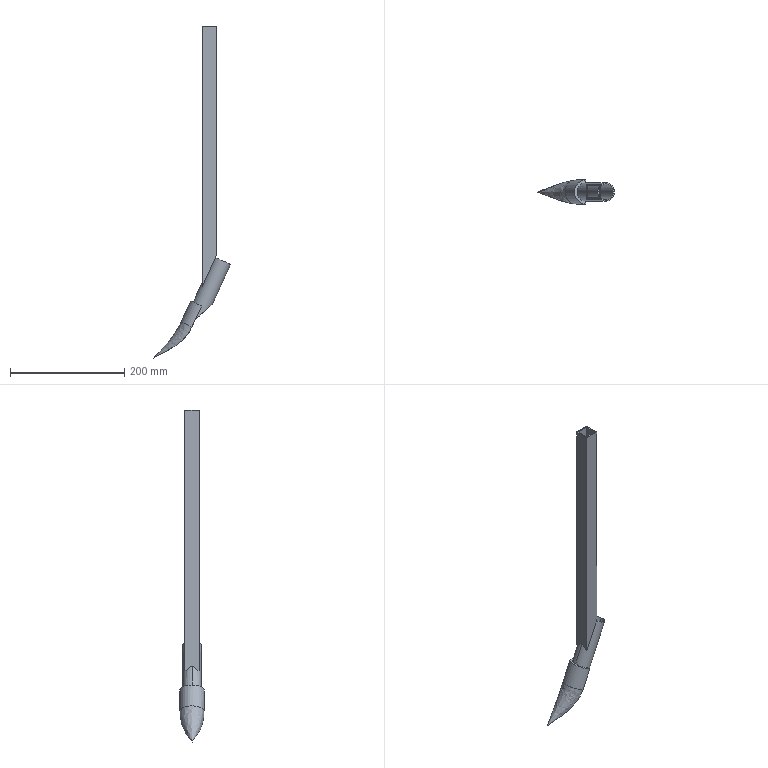Part | SolidWorks | features ICE 5, Blend 1, Extrusion 1 | 1 solid | 31 faces | box 134.332 x 42 x 580 mm | volume 122750 mm3 | plane 19 | cylinder 8 | spline 4 | commonest cylinder face diameters 32 x5 28 x2 42 x1
STEP:
#1=CARTESIAN_POINT('',(2.036,0.,-33.269));
#2=VERTEX_POINT('',#1);
#3=CARTESIAN_POINT('',(-50.61,0.,-81.426));
#4=VERTEX_POINT('',#3);
#5=CARTESIAN_POINT('',(2.036,0.,-33.269));
#6=CARTESIAN_POINT('',(2.036,-28.,-33.269));
#7=CARTESIAN_POINT('',(-50.61,-28.,-81.426));
#8=CARTESIAN_POINT('',(-50.61,0.,-81.426));
#9=(BOUNDED_CURVE()B_SPLINE_CURVE(3,(#5,#6,#7,#8),.UNSPECIFIED.,.F.,.F.)B_SPLINE_CURVE_WITH_KNOTS((4,4),(0.,3.142),.UNSPECIFIED.)CURVE()GEOMETRIC_REPRESENTATION_ITEM()RATIONAL_B_SPLINE_CURVE((1.,0.3333,0.3333,1.))REPRESENTATION_ITEM(''));
#10=EDGE_CURVE('',#2,#4,#9,.T.);
#11=ORIENTED_EDGE('',*,*,#10,.T.);
#12=CARTESIAN_POINT('',(-12.5,0.,2.417));
#13=VERTEX_POINT('',#12);
#14=CARTESIAN_POINT('',(-52.55,0.,-85.693));
#15=DIRECTION('',(0.4138,0.,0.9104));
#16=VECTOR('',#15,1000.);
#17=LINE('',#14,#16);
#18=EDGE_CURVE('',#4,#13,#17,.T.);
#19=ORIENTED_EDGE('',*,*,#18,.T.);
#20=CARTESIAN_POINT('',(-12.5,-3.14,1.555));
#21=VERTEX_POINT('',#20);
#22=CARTESIAN_POINT('',(-12.5,0.,2.417));
#23=CARTESIAN_POINT('',(-12.5,-1.058,2.417));
#24=CARTESIAN_POINT('',(-12.5,-2.109,2.128));
#25=CARTESIAN_POINT('',(-12.5,-3.14,1.555));
#26=(BOUNDED_CURVE()B_SPLINE_CURVE(3,(#22,#23,#24,#25),.UNSPECIFIED.,.F.,.T.)B_SPLINE_CURVE_WITH_KNOTS((4,4),(0.,0.2262),.UNSPECIFIED.)CURVE()GEOMETRIC_REPRESENTATION_ITEM()RATIONAL_B_SPLINE_CURVE((1.,0.9957,0.9957,1.))REPRESENTATION_ITEM(''));
#27=EDGE_CURVE('',#13,#21,#26,.T.);
#28=ORIENTED_EDGE('',*,*,#27,.T.);
#29=CARTESIAN_POINT('',(-11.914,-5.196,1.288));
#30=VERTEX_POINT('',#29);
#31=CARTESIAN_POINT('',(-0.07961,0.,-4.091));
#32=DIRECTION('',(-0.4138,0.,-0.9104));
#33=DIRECTION('',(-0.9104,0.,0.4138));
#34=AXIS2_PLACEMENT_3D('',#31,#32,#33);
#35=CIRCLE('',#34,14.);
#36=EDGE_CURVE('',#30,#21,#35,.T.);
#37=ORIENTED_EDGE('',*,*,#36,.F.);
#38=CARTESIAN_POINT('',(-10.5,-5.196,4.4));
#39=VERTEX_POINT('',#38);
#40=CARTESIAN_POINT('',(-51.639,-5.196,-86.107));
#41=DIRECTION('',(0.4138,0.,0.9104));
#42=VECTOR('',#41,1000.);
#43=LINE('',#40,#42);
#44=EDGE_CURVE('',#30,#39,#43,.T.);
#45=ORIENTED_EDGE('',*,*,#44,.T.);
#46=CARTESIAN_POINT('',(-10.5,0.,6.817));
#47=VERTEX_POINT('',#46);
#48=CARTESIAN_POINT('',(-10.5,0.,6.817));
#49=CARTESIAN_POINT('',(-10.5,-1.785,6.817));
#50=CARTESIAN_POINT('',(-10.5,-3.538,6.001));
#51=CARTESIAN_POINT('',(-10.5,-5.196,4.4));
#52=(BOUNDED_CURVE()B_SPLINE_CURVE(3,(#48,#49,#50,#51),.UNSPECIFIED.,.F.,.F.)B_SPLINE_CURVE_WITH_KNOTS((4,4),(0.,0.3803),.UNSPECIFIED.)CURVE()GEOMETRIC_REPRESENTATION_ITEM()RATIONAL_B_SPLINE_CURVE((1.,0.988,0.988,1.))REPRESENTATION_ITEM(''));
#53=EDGE_CURVE('',#47,#39,#52,.T.);
#54=ORIENTED_EDGE('',*,*,#53,.F.);
#55=CARTESIAN_POINT('',(9.521,0.,50.862));
#56=VERTEX_POINT('',#55);
#57=CARTESIAN_POINT('',(-52.55,0.,-85.693));
#58=DIRECTION('',(0.4138,0.,0.9104));
#59=VECTOR('',#58,1000.);
#60=LINE('',#57,#59);
#61=EDGE_CURVE('',#47,#56,#60,.T.);
#62=ORIENTED_EDGE('',*,*,#61,.T.);
#63=CARTESIAN_POINT('',(35.011,0.,39.275));
#64=VERTEX_POINT('',#63);
#65=CARTESIAN_POINT('',(22.266,0.,45.069));
#66=DIRECTION('',(0.4138,0.,0.9104));
#67=DIRECTION('',(0.9104,0.,-0.4138));
#68=AXIS2_PLACEMENT_3D('',#65,#66,#67);
#69=CIRCLE('',#68,14.);
#70=EDGE_CURVE('',#56,#64,#69,.T.);
#71=ORIENTED_EDGE('',*,*,#70,.T.);
#72=CARTESIAN_POINT('',(-27.06,0.,-97.279));
#73=DIRECTION('',(0.4138,0.,0.9104));
#74=VECTOR('',#73,1000.);
#75=LINE('',#72,#74);
#76=EDGE_CURVE('',#2,#64,#75,.T.);
#77=ORIENTED_EDGE('',*,*,#76,.F.);
#78=EDGE_LOOP('',(#11,#19,#28,#37,#45,#54,#62,#71,#77));
#79=FACE_OUTER_BOUND('',#78,.T.);
#80=CARTESIAN_POINT('',(-39.805,0.,-91.486));
#81=DIRECTION('',(0.4138,0.,0.9104));
#82=DIRECTION('',(0.9104,0.,-0.4138));
#83=AXIS2_PLACEMENT_3D('',#80,#81,#82);
#84=CYLINDRICAL_SURFACE('',#83,14.);
#85=ADVANCED_FACE('',(#79),#84,.F.);
#86=CARTESIAN_POINT('',(-28.301,0.,-27.512));
#87=VERTEX_POINT('',#86);
#88=CARTESIAN_POINT('',(-13.735,16.,-34.133));
#89=VERTEX_POINT('',#88);
#90=CARTESIAN_POINT('',(-13.735,0.,-34.133));
#91=DIRECTION('',(-0.4138,0.,-0.9104));
#92=DIRECTION('',(0.9104,0.,-0.4138));
#93=AXIS2_PLACEMENT_3D('',#90,#91,#92);
#94=CIRCLE('',#93,16.);
#95=EDGE_CURVE('',#87,#89,#94,.T.);
#96=ORIENTED_EDGE('',*,*,#95,.F.);
#97=CARTESIAN_POINT('',(-12.5,0.,7.25));
#98=VERTEX_POINT('',#97);
#99=CARTESIAN_POINT('',(-54.371,0.,-84.865));
#100=DIRECTION('',(0.4138,0.,0.9104));
#101=VECTOR('',#100,1000.);
#102=LINE('',#99,#101);
#103=EDGE_CURVE('',#87,#98,#102,.T.);
#104=ORIENTED_EDGE('',*,*,#103,.T.);
#105=CARTESIAN_POINT('',(-12.5,9.327,0.));
#106=VERTEX_POINT('',#105);
#107=CARTESIAN_POINT('',(-12.5,9.327,0.));
#108=CARTESIAN_POINT('',(-12.5,6.586,4.753));
#109=CARTESIAN_POINT('',(-12.5,3.374,7.25));
#110=CARTESIAN_POINT('',(-12.5,0.,7.25));
#111=(BOUNDED_CURVE()B_SPLINE_CURVE(3,(#107,#108,#109,#110),.UNSPECIFIED.,.F.,.F.)B_SPLINE_CURVE_WITH_KNOTS((4,4),(5.661,6.283),.UNSPECIFIED.)CURVE()GEOMETRIC_REPRESENTATION_ITEM()RATIONAL_B_SPLINE_CURVE((1.,0.968,0.968,1.))REPRESENTATION_ITEM(''));
#112=EDGE_CURVE('',#106,#98,#111,.T.);
#113=ORIENTED_EDGE('',*,*,#112,.F.);
#114=CARTESIAN_POINT('',(-10.5,9.327,4.4));
#115=VERTEX_POINT('',#114);
#116=CARTESIAN_POINT('',(-51.639,9.327,-86.107));
#117=DIRECTION('',(-0.4138,0.,-0.9104));
#118=VECTOR('',#117,1000.);
#119=LINE('',#116,#118);
#120=EDGE_CURVE('',#115,#106,#119,.T.);
#121=ORIENTED_EDGE('',*,*,#120,.F.);
#122=CARTESIAN_POINT('',(-10.5,0.,11.65));
#123=VERTEX_POINT('',#122);
#124=CARTESIAN_POINT('',(-10.5,9.327,4.4));
#125=CARTESIAN_POINT('',(-10.5,6.586,9.153));
#126=CARTESIAN_POINT('',(-10.5,3.374,11.65));
#127=CARTESIAN_POINT('',(-10.5,0.,11.65));
#128=(BOUNDED_CURVE()B_SPLINE_CURVE(3,(#124,#125,#126,#127),.UNSPECIFIED.,.F.,.F.)B_SPLINE_CURVE_WITH_KNOTS((4,4),(5.661,6.283),.UNSPECIFIED.)CURVE()GEOMETRIC_REPRESENTATION_ITEM()RATIONAL_B_SPLINE_CURVE((1.,0.968,0.968,1.))REPRESENTATION_ITEM(''));
#129=EDGE_CURVE('',#115,#123,#128,.T.);
#130=ORIENTED_EDGE('',*,*,#129,.T.);
#131=CARTESIAN_POINT('',(7.7,0.,51.69));
#132=VERTEX_POINT('',#131);
#133=CARTESIAN_POINT('',(-54.371,0.,-84.865));
#134=DIRECTION('',(0.4138,0.,0.9104));
#135=VECTOR('',#134,1000.);
#136=LINE('',#133,#135);
#137=EDGE_CURVE('',#123,#132,#136,.T.);
#138=ORIENTED_EDGE('',*,*,#137,.T.);
#139=CARTESIAN_POINT('',(36.832,0.,38.448));
#140=VERTEX_POINT('',#139);
#141=CARTESIAN_POINT('',(22.266,0.,45.069));
#142=DIRECTION('',(0.4138,0.,0.9104));
#143=DIRECTION('',(0.9104,0.,-0.4138));
#144=AXIS2_PLACEMENT_3D('',#141,#142,#143);
#145=CIRCLE('',#144,16.);
#146=EDGE_CURVE('',#140,#132,#145,.T.);
#147=ORIENTED_EDGE('',*,*,#146,.F.);
#148=CARTESIAN_POINT('',(5.796,0.,-29.83));
#149=VERTEX_POINT('',#148);
#150=CARTESIAN_POINT('',(-25.239,0.,-98.107));
#151=DIRECTION('',(0.4138,0.,0.9104));
#152=VECTOR('',#151,1000.);
#153=LINE('',#150,#152);
#154=EDGE_CURVE('',#149,#140,#153,.T.);
#155=ORIENTED_EDGE('',*,*,#154,.F.);
#156=CARTESIAN_POINT('',(-24.287,16.,-57.347));
#157=VERTEX_POINT('',#156);
#158=CARTESIAN_POINT('',(-24.287,16.,-57.347));
#159=CARTESIAN_POINT('',(-6.665,16.,-41.228));
#160=CARTESIAN_POINT('',(5.796,9.373,-29.83));
#161=CARTESIAN_POINT('',(5.796,0.,-29.83));
#162=(BOUNDED_CURVE()B_SPLINE_CURVE(3,(#158,#159,#160,#161),.UNSPECIFIED.,.F.,.F.)B_SPLINE_CURVE_WITH_KNOTS((4,4),(4.712,6.283),.UNSPECIFIED.)CURVE()GEOMETRIC_REPRESENTATION_ITEM()RATIONAL_B_SPLINE_CURVE((1.,0.8047,0.8047,1.))REPRESENTATION_ITEM(''));
#163=EDGE_CURVE('',#157,#149,#162,.T.);
#164=ORIENTED_EDGE('',*,*,#163,.F.);
#165=CARTESIAN_POINT('',(-30.287,16.,-70.548));
#166=DIRECTION('',(0.4138,0.,0.9104));
#167=VECTOR('',#166,1000.);
#168=LINE('',#165,#167);
#169=EDGE_CURVE('',#157,#89,#168,.T.);
#170=ORIENTED_EDGE('',*,*,#169,.T.);
#171=EDGE_LOOP('',(#96,#104,#113,#121,#130,#138,#147,#155,#164,#170));
#172=FACE_OUTER_BOUND('',#171,.T.);
#173=CARTESIAN_POINT('',(-39.805,0.,-91.486));
#174=DIRECTION('',(0.4138,0.,0.9104));
#175=DIRECTION('',(0.9104,0.,-0.4138));
#176=AXIS2_PLACEMENT_3D('',#173,#174,#175);
#177=CYLINDRICAL_SURFACE('',#176,16.);
#178=ADVANCED_FACE('',(#172),#177,.T.);
#179=CARTESIAN_POINT('',(-37.266,14.434,-69.22));
#180=VERTEX_POINT('',#179);
#181=CARTESIAN_POINT('',(-36.571,14.434,-67.691));
#182=VERTEX_POINT('',#181);
#183=CARTESIAN_POINT('',(-37.266,14.434,-69.22));
#184=CARTESIAN_POINT('',(-37.035,14.434,-68.711));
#185=CARTESIAN_POINT('',(-36.803,14.434,-68.202));
#186=CARTESIAN_POINT('',(-36.571,14.434,-67.691));
#187=B_SPLINE_CURVE_WITH_KNOTS('',3,(#183,#184,#185,#186),.UNSPECIFIED.,.F.,.F.,(4,4),(0.8196,1.),.UNSPECIFIED.);
#188=EDGE_CURVE('',#180,#182,#187,.T.);
#189=ORIENTED_EDGE('',*,*,#188,.F.);
#190=CARTESIAN_POINT('',(-37.266,-14.434,-69.22));
#191=VERTEX_POINT('',#190);
#192=CARTESIAN_POINT('',(-37.266,-14.434,-69.22));
#193=CARTESIAN_POINT('',(-63.552,-7.748,-93.264));
#194=CARTESIAN_POINT('',(-63.552,7.748,-93.264));
#195=CARTESIAN_POINT('',(-37.266,14.434,-69.22));
#196=(BOUNDED_CURVE()B_SPLINE_CURVE(3,(#192,#193,#194,#195),.UNSPECIFIED.,.F.,.T.)B_SPLINE_CURVE_WITH_KNOTS((4,4),(2.017,4.266),.UNSPECIFIED.)CURVE()GEOMETRIC_REPRESENTATION_ITEM()RATIONAL_B_SPLINE_CURVE((1.,0.621,0.621,1.))REPRESENTATION_ITEM(''));
#197=EDGE_CURVE('',#191,#180,#196,.T.);
#198=ORIENTED_EDGE('',*,*,#197,.F.);
#199=CARTESIAN_POINT('',(-36.571,-14.434,-67.691));
#200=VERTEX_POINT('',#199);
#201=CARTESIAN_POINT('',(-37.266,-14.434,-69.22));
#202=CARTESIAN_POINT('',(-37.034,-14.434,-68.71));
#203=CARTESIAN_POINT('',(-36.803,-14.434,-68.201));
#204=CARTESIAN_POINT('',(-36.571,-14.434,-67.691));
#205=B_SPLINE_CURVE_WITH_KNOTS('',3,(#201,#202,#203,#204),.UNSPECIFIED.,.F.,.F.,(4,4),(0.8182,1.),.UNSPECIFIED.);
#206=EDGE_CURVE('',#191,#200,#205,.T.);
#207=ORIENTED_EDGE('',*,*,#206,.T.);
#208=CARTESIAN_POINT('',(-30.287,0.,-70.548));
#209=DIRECTION('',(0.4138,0.,0.9104));
#210=DIRECTION('',(-0.9104,0.,0.4138));
#211=AXIS2_PLACEMENT_3D('',#208,#209,#210);
#212=CIRCLE('',#211,16.);
#213=EDGE_CURVE('',#182,#200,#212,.T.);
#214=ORIENTED_EDGE('',*,*,#213,.F.);
#215=EDGE_LOOP('',(#189,#198,#207,#214));
#216=FACE_OUTER_BOUND('',#215,.T.);
#217=CARTESIAN_POINT('',(-39.805,0.,-91.486));
#218=DIRECTION('',(0.4138,0.,0.9104));
#219=DIRECTION('',(0.9104,0.,-0.4138));
#220=AXIS2_PLACEMENT_3D('',#217,#218,#219);
#221=CYLINDRICAL_SURFACE('',#220,16.);
#222=ADVANCED_FACE('',(#216),#221,.T.);
#223=CARTESIAN_POINT('',(-11.914,5.196,1.288));
#224=VERTEX_POINT('',#223);
#225=CARTESIAN_POINT('',(-11.914,-202.5,1.288));
#226=DIRECTION('',(0.,-1.,0.));
#227=VECTOR('',#226,1000.);
#228=LINE('',#225,#227);
#229=EDGE_CURVE('',#224,#30,#228,.T.);
#230=ORIENTED_EDGE('',*,*,#229,.F.);
#231=CARTESIAN_POINT('',(-10.5,5.196,4.4));
#232=VERTEX_POINT('',#231);
#233=CARTESIAN_POINT('',(-51.639,5.196,-86.107));
#234=DIRECTION('',(-0.4138,0.,-0.9104));
#235=VECTOR('',#234,1000.);
#236=LINE('',#233,#235);
#237=EDGE_CURVE('',#232,#224,#236,.T.);
#238=ORIENTED_EDGE('',*,*,#237,.F.);
#239=CARTESIAN_POINT('',(-10.5,-10.5,4.4));
#240=DIRECTION('',(0.,-1.,0.));
#241=VECTOR('',#240,1000.);
#242=LINE('',#239,#241);
#243=EDGE_CURVE('',#232,#39,#242,.T.);
#244=ORIENTED_EDGE('',*,*,#243,.T.);
#245=ORIENTED_EDGE('',*,*,#44,.F.);
#246=EDGE_LOOP('',(#230,#238,#244,#245));
#247=FACE_OUTER_BOUND('',#246,.T.);
#248=CARTESIAN_POINT('',(-12.5,-202.5,0.));
#249=DIRECTION('',(-0.9104,0.,0.4138));
#250=DIRECTION('',(0.4138,0.,0.9104));
#251=AXIS2_PLACEMENT_3D('',#248,#249,#250);
#252=PLANE('',#251);
#253=ADVANCED_FACE('',(#247),#252,.F.);
#254=CARTESIAN_POINT('',(-12.5,3.14,1.555));
#255=VERTEX_POINT('',#254);
#256=CARTESIAN_POINT('',(-12.5,-12.5,1.555));
#257=DIRECTION('',(0.,1.,0.));
#258=VECTOR('',#257,1000.);
#259=LINE('',#256,#258);
#260=EDGE_CURVE('',#21,#255,#259,.T.);
#261=ORIENTED_EDGE('',*,*,#260,.F.);
#262=ORIENTED_EDGE('',*,*,#27,.F.);
#263=CARTESIAN_POINT('',(-12.5,3.14,1.555));
#264=CARTESIAN_POINT('',(-12.5,2.109,2.128));
#265=CARTESIAN_POINT('',(-12.5,1.058,2.417));
#266=CARTESIAN_POINT('',(-12.5,0.,2.417));
#267=(BOUNDED_CURVE()B_SPLINE_CURVE(3,(#263,#264,#265,#266),.UNSPECIFIED.,.F.,.F.)B_SPLINE_CURVE_WITH_KNOTS((4,4),(6.057,6.283),.UNSPECIFIED.)CURVE()GEOMETRIC_REPRESENTATION_ITEM()RATIONAL_B_SPLINE_CURVE((1.,0.9957,0.9957,1.))REPRESENTATION_ITEM(''));
#268=EDGE_CURVE('',#255,#13,#267,.T.);
#269=ORIENTED_EDGE('',*,*,#268,.F.);
#270=EDGE_LOOP('',(#261,#262,#269));
#271=FACE_OUTER_BOUND('',#270,.T.);
#272=CARTESIAN_POINT('',(-12.5,-12.5,455.));
#273=DIRECTION('',(1.,0.,0.));
#274=DIRECTION('',(0.,0.,-1.));
#275=AXIS2_PLACEMENT_3D('',#272,#273,#274);
#276=PLANE('',#275);
#277=ADVANCED_FACE('',(#271),#276,.F.);
#278=CARTESIAN_POINT('',(-12.5,12.5,455.));
#279=VERTEX_POINT('',#278);
#280=CARTESIAN_POINT('',(-12.5,-12.5,455.));
#281=VERTEX_POINT('',#280);
#282=CARTESIAN_POINT('',(-12.5,-12.5,455.));
#283=DIRECTION('',(0.,-1.,0.));
#284=VECTOR('',#283,1000.);
#285=LINE('',#282,#284);
#286=EDGE_CURVE('',#279,#281,#285,.T.);
#287=ORIENTED_EDGE('',*,*,#286,.T.);
#288=CARTESIAN_POINT('',(12.5,-12.5,455.));
#289=VERTEX_POINT('',#288);
#290=CARTESIAN_POINT('',(12.5,-12.5,455.));
#291=DIRECTION('',(1.,0.,0.));
#292=VECTOR('',#291,1000.);
#293=LINE('',#290,#292);
#294=EDGE_CURVE('',#281,#289,#293,.T.);
#295=ORIENTED_EDGE('',*,*,#294,.T.);
#296=CARTESIAN_POINT('',(12.5,12.5,455.));
#297=VERTEX_POINT('',#296);
#298=CARTESIAN_POINT('',(12.5,-12.5,455.));
#299=DIRECTION('',(0.,1.,0.));
#300=VECTOR('',#299,1000.);
#301=LINE('',#298,#300);
#302=EDGE_CURVE('',#289,#297,#301,.T.);
#303=ORIENTED_EDGE('',*,*,#302,.T.);
#304=CARTESIAN_POINT('',(12.5,12.5,455.));
#305=DIRECTION('',(-1.,0.,0.));
#306=VECTOR('',#305,1000.);
#307=LINE('',#304,#306);
#308=EDGE_CURVE('',#297,#279,#307,.T.);
#309=ORIENTED_EDGE('',*,*,#308,.T.);
#310=EDGE_LOOP('',(#287,#295,#303,#309));
#311=FACE_OUTER_BOUND('',#310,.T.);
#312=CARTESIAN_POINT('',(-10.5,-10.5,455.));
#313=VERTEX_POINT('',#312);
#314=CARTESIAN_POINT('',(10.5,-10.5,455.));
#315=VERTEX_POINT('',#314);
#316=CARTESIAN_POINT('',(10.5,-10.5,455.));
#317=DIRECTION('',(1.,0.,0.));
#318=VECTOR('',#317,1000.);
#319=LINE('',#316,#318);
#320=EDGE_CURVE('',#313,#315,#319,.T.);
#321=ORIENTED_EDGE('',*,*,#320,.F.);
#322=CARTESIAN_POINT('',(-10.5,10.5,455.));
#323=VERTEX_POINT('',#322);
#324=CARTESIAN_POINT('',(-10.5,-10.5,455.));
#325=DIRECTION('',(0.,-1.,0.));
#326=VECTOR('',#325,1000.);
#327=LINE('',#324,#326);
#328=EDGE_CURVE('',#323,#313,#327,.T.);
#329=ORIENTED_EDGE('',*,*,#328,.F.);
#330=CARTESIAN_POINT('',(10.5,10.5,455.));
#331=VERTEX_POINT('',#330);
#332=CARTESIAN_POINT('',(10.5,10.5,455.));
#333=DIRECTION('',(-1.,0.,0.));
#334=VECTOR('',#333,1000.);
#335=LINE('',#332,#334);
#336=EDGE_CURVE('',#331,#323,#335,.T.);
#337=ORIENTED_EDGE('',*,*,#336,.F.);
#338=CARTESIAN_POINT('',(10.5,-10.5,455.));
#339=DIRECTION('',(0.,1.,0.));
#340=VECTOR('',#339,1000.);
#341=LINE('',#338,#340);
#342=EDGE_CURVE('',#315,#331,#341,.T.);
#343=ORIENTED_EDGE('',*,*,#342,.F.);
#344=EDGE_LOOP('',(#321,#329,#337,#343));
#345=FACE_BOUND('',#344,.T.);
#346=CARTESIAN_POINT('',(0.,0.,455.));
#347=DIRECTION('',(0.,0.,1.));
#348=DIRECTION('',(1.,0.,0.));
#349=AXIS2_PLACEMENT_3D('',#346,#347,#348);
#350=PLANE('',#349);
#351=ADVANCED_FACE('',(#311,#345),#350,.T.);
#352=CARTESIAN_POINT('',(-12.5,12.5,0.));
#353=VERTEX_POINT('',#352);
#354=CARTESIAN_POINT('',(-12.5,-12.5,0.));
#355=DIRECTION('',(0.,-1.,0.));
#356=VECTOR('',#355,1000.);
#357=LINE('',#354,#356);
#358=EDGE_CURVE('',#353,#106,#357,.T.);
#359=ORIENTED_EDGE('',*,*,#358,.T.);
#360=ORIENTED_EDGE('',*,*,#112,.T.);
#361=CARTESIAN_POINT('',(-12.5,-9.327,0.));
#362=VERTEX_POINT('',#361);
#363=CARTESIAN_POINT('',(-12.5,0.,7.25));
#364=CARTESIAN_POINT('',(-12.5,-3.374,7.25));
#365=CARTESIAN_POINT('',(-12.5,-6.586,4.753));
#366=CARTESIAN_POINT('',(-12.5,-9.327,0.));
#367=(BOUNDED_CURVE()B_SPLINE_CURVE(3,(#363,#364,#365,#366),.UNSPECIFIED.,.F.,.T.)B_SPLINE_CURVE_WITH_KNOTS((4,4),(0.,0.6224),.UNSPECIFIED.)CURVE()GEOMETRIC_REPRESENTATION_ITEM()RATIONAL_B_SPLINE_CURVE((1.,0.968,0.968,1.))REPRESENTATION_ITEM(''));
#368=EDGE_CURVE('',#98,#362,#367,.T.);
#369=ORIENTED_EDGE('',*,*,#368,.T.);
#370=CARTESIAN_POINT('',(-12.5,-12.5,0.));
#371=VERTEX_POINT('',#370);
#372=CARTESIAN_POINT('',(-12.5,-12.5,0.));
#373=DIRECTION('',(0.,-1.,0.));
#374=VECTOR('',#373,1000.);
#375=LINE('',#372,#374);
#376=EDGE_CURVE('',#362,#371,#375,.T.);
#377=ORIENTED_EDGE('',*,*,#376,.T.);
#378=CARTESIAN_POINT('',(-12.5,-12.5,455.));
#379=DIRECTION('',(0.,0.,-1.));
#380=VECTOR('',#379,1000.);
#381=LINE('',#378,#380);
#382=EDGE_CURVE('',#281,#371,#381,.T.);
#383=ORIENTED_EDGE('',*,*,#382,.F.);
#384=ORIENTED_EDGE('',*,*,#286,.F.);
#385=CARTESIAN_POINT('',(-12.5,12.5,455.));
#386=DIRECTION('',(0.,0.,-1.));
#387=VECTOR('',#386,1000.);
#388=LINE('',#385,#387);
#389=EDGE_CURVE('',#279,#353,#388,.T.);
#390=ORIENTED_EDGE('',*,*,#389,.T.);
#391=EDGE_LOOP('',(#359,#360,#369,#377,#383,#384,#390));
#392=FACE_OUTER_BOUND('',#391,.T.);
#393=CARTESIAN_POINT('',(-12.5,-12.5,455.));
#394=DIRECTION('',(1.,0.,0.));
#395=DIRECTION('',(0.,0.,-1.));
#396=AXIS2_PLACEMENT_3D('',#393,#394,#395);
#397=PLANE('',#396);
#398=ADVANCED_FACE('',(#392),#397,.F.);
#399=ORIENTED_EDGE('',*,*,#382,.T.);
#400=CARTESIAN_POINT('',(12.5,-12.5,55.));
#401=VERTEX_POINT('',#400);
#402=CARTESIAN_POINT('',(163.185,-12.5,386.507));
#403=DIRECTION('',(0.4138,0.,0.9104));
#404=VECTOR('',#403,1000.);
#405=LINE('',#402,#404);
#406=EDGE_CURVE('',#371,#401,#405,.T.);
#407=ORIENTED_EDGE('',*,*,#406,.T.);
#408=CARTESIAN_POINT('',(12.5,-12.5,455.));
#409=DIRECTION('',(0.,0.,-1.));
#410=VECTOR('',#409,1000.);
#411=LINE('',#408,#410);
#412=EDGE_CURVE('',#289,#401,#411,.T.);
#413=ORIENTED_EDGE('',*,*,#412,.F.);
#414=ORIENTED_EDGE('',*,*,#294,.F.);
#415=EDGE_LOOP('',(#399,#407,#413,#414));
#416=FACE_OUTER_BOUND('',#415,.T.);
#417=CARTESIAN_POINT('',(12.5,-12.5,455.));
#418=DIRECTION('',(0.,1.,0.));
#419=DIRECTION('',(-1.,0.,0.));
#420=AXIS2_PLACEMENT_3D('',#417,#418,#419);
#421=PLANE('',#420);
#422=ADVANCED_FACE('',(#416),#421,.F.);
#423=ORIENTED_EDGE('',*,*,#412,.T.);
#424=CARTESIAN_POINT('',(12.5,12.5,55.));
#425=VERTEX_POINT('',#424);
#426=CARTESIAN_POINT('',(12.5,-202.5,55.));
#427=DIRECTION('',(0.,1.,0.));
#428=VECTOR('',#427,1000.);
#429=LINE('',#426,#428);
#430=EDGE_CURVE('',#401,#425,#429,.T.);
#431=ORIENTED_EDGE('',*,*,#430,.T.);
#432=CARTESIAN_POINT('',(12.5,12.5,455.));
#433=DIRECTION('',(0.,0.,-1.));
#434=VECTOR('',#433,1000.);
#435=LINE('',#432,#434);
#436=EDGE_CURVE('',#297,#425,#435,.T.);
#437=ORIENTED_EDGE('',*,*,#436,.F.);
#438=ORIENTED_EDGE('',*,*,#302,.F.);
#439=EDGE_LOOP('',(#423,#431,#437,#438));
#440=FACE_OUTER_BOUND('',#439,.T.);
#441=CARTESIAN_POINT('',(12.5,-12.5,455.));
#442=DIRECTION('',(-1.,0.,0.));
#443=DIRECTION('',(0.,0.,1.));
#444=AXIS2_PLACEMENT_3D('',#441,#442,#443);
#445=PLANE('',#444);
#446=ADVANCED_FACE('',(#440),#445,.F.);
#447=ORIENTED_EDGE('',*,*,#436,.T.);
#448=CARTESIAN_POINT('',(-12.5,12.5,0.));
#449=DIRECTION('',(0.4138,0.,0.9104));
#450=VECTOR('',#449,1000.);
#451=LINE('',#448,#450);
#452=EDGE_CURVE('',#353,#425,#451,.T.);
#453=ORIENTED_EDGE('',*,*,#452,.F.);
#454=ORIENTED_EDGE('',*,*,#389,.F.);
#455=ORIENTED_EDGE('',*,*,#308,.F.);
#456=EDGE_LOOP('',(#447,#453,#454,#455));
#457=FACE_OUTER_BOUND('',#456,.T.);
#458=CARTESIAN_POINT('',(12.5,12.5,455.));
#459=DIRECTION('',(0.,-1.,0.));
#460=DIRECTION('',(1.,0.,0.));
#461=AXIS2_PLACEMENT_3D('',#458,#459,#460);
#462=PLANE('',#461);
#463=ADVANCED_FACE('',(#457),#462,.F.);
#464=ORIENTED_EDGE('',*,*,#129,.F.);
#465=CARTESIAN_POINT('',(-10.5,10.5,4.4));
#466=VERTEX_POINT('',#465);
#467=CARTESIAN_POINT('',(-10.5,-10.5,4.4));
#468=DIRECTION('',(0.,-1.,0.));
#469=VECTOR('',#468,1000.);
#470=LINE('',#467,#469);
#471=EDGE_CURVE('',#466,#115,#470,.T.);
#472=ORIENTED_EDGE('',*,*,#471,.F.);
#473=CARTESIAN_POINT('',(-10.5,10.5,455.));
#474=DIRECTION('',(0.,0.,-1.));
#475=VECTOR('',#474,1000.);
#476=LINE('',#473,#475);
#477=EDGE_CURVE('',#323,#466,#476,.T.);
#478=ORIENTED_EDGE('',*,*,#477,.F.);
#479=ORIENTED_EDGE('',*,*,#328,.T.);
#480=CARTESIAN_POINT('',(-10.5,-10.5,4.4));
#481=VERTEX_POINT('',#480);
#482=CARTESIAN_POINT('',(-10.5,-10.5,455.));
#483=DIRECTION('',(0.,0.,-1.));
#484=VECTOR('',#483,1000.);
#485=LINE('',#482,#484);
#486=EDGE_CURVE('',#313,#481,#485,.T.);
#487=ORIENTED_EDGE('',*,*,#486,.T.);
#488=CARTESIAN_POINT('',(-10.5,-9.327,4.4));
#489=VERTEX_POINT('',#488);
#490=CARTESIAN_POINT('',(-10.5,-10.5,4.4));
#491=DIRECTION('',(0.,-1.,0.));
#492=VECTOR('',#491,1000.);
#493=LINE('',#490,#492);
#494=EDGE_CURVE('',#489,#481,#493,.T.);
#495=ORIENTED_EDGE('',*,*,#494,.F.);
#496=CARTESIAN_POINT('',(-10.5,0.,11.65));
#497=CARTESIAN_POINT('',(-10.5,-3.374,11.65));
#498=CARTESIAN_POINT('',(-10.5,-6.586,9.153));
#499=CARTESIAN_POINT('',(-10.5,-9.327,4.4));
#500=(BOUNDED_CURVE()B_SPLINE_CURVE(3,(#496,#497,#498,#499),.UNSPECIFIED.,.F.,.F.)B_SPLINE_CURVE_WITH_KNOTS((4,4),(0.,0.6224),.UNSPECIFIED.)CURVE()GEOMETRIC_REPRESENTATION_ITEM()RATIONAL_B_SPLINE_CURVE((1.,0.968,0.968,1.))REPRESENTATION_ITEM(''));
#501=EDGE_CURVE('',#123,#489,#500,.T.);
#502=ORIENTED_EDGE('',*,*,#501,.F.);
#503=EDGE_LOOP('',(#464,#472,#478,#479,#487,#495,#502));
#504=FACE_OUTER_BOUND('',#503,.T.);
#505=CARTESIAN_POINT('',(-10.5,-10.5,455.));
#506=DIRECTION('',(1.,0.,0.));
#507=DIRECTION('',(0.,1.,0.));
#508=AXIS2_PLACEMENT_3D('',#505,#506,#507);
#509=PLANE('',#508);
#510=ADVANCED_FACE('',(#504),#509,.T.);
#511=CARTESIAN_POINT('',(10.5,-10.5,50.6));
#512=VERTEX_POINT('',#511);
#513=CARTESIAN_POINT('',(162.842,-10.5,385.753));
#514=DIRECTION('',(0.4138,0.,0.9104));
#515=VECTOR('',#514,1000.);
#516=LINE('',#513,#515);
#517=EDGE_CURVE('',#481,#512,#516,.T.);
#518=ORIENTED_EDGE('',*,*,#517,.F.);
#519=ORIENTED_EDGE('',*,*,#486,.F.);
#520=ORIENTED_EDGE('',*,*,#320,.T.);
#521=CARTESIAN_POINT('',(10.5,-10.5,455.));
#522=DIRECTION('',(0.,0.,-1.));
#523=VECTOR('',#522,1000.);
#524=LINE('',#521,#523);
#525=EDGE_CURVE('',#315,#512,#524,.T.);
#526=ORIENTED_EDGE('',*,*,#525,.T.);
#527=EDGE_LOOP('',(#518,#519,#520,#526));
#528=FACE_OUTER_BOUND('',#527,.T.);
#529=CARTESIAN_POINT('',(10.5,-10.5,455.));
#530=DIRECTION('',(0.,1.,0.));
#531=DIRECTION('',(0.,0.,1.));
#532=AXIS2_PLACEMENT_3D('',#529,#530,#531);
#533=PLANE('',#532);
#534=ADVANCED_FACE('',(#528),#533,.T.);
#535=CARTESIAN_POINT('',(10.5,10.5,50.6));
#536=VERTEX_POINT('',#535);
#537=CARTESIAN_POINT('',(10.5,-10.5,50.6));
#538=DIRECTION('',(0.,1.,0.));
#539=VECTOR('',#538,1000.);
#540=LINE('',#537,#539);
#541=EDGE_CURVE('',#512,#536,#540,.T.);
#542=ORIENTED_EDGE('',*,*,#541,.F.);
#543=ORIENTED_EDGE('',*,*,#525,.F.);
#544=ORIENTED_EDGE('',*,*,#342,.T.);
#545=CARTESIAN_POINT('',(10.5,10.5,455.));
#546=DIRECTION('',(0.,0.,-1.));
#547=VECTOR('',#546,1000.);
#548=LINE('',#545,#547);
#549=EDGE_CURVE('',#331,#536,#548,.T.);
#550=ORIENTED_EDGE('',*,*,#549,.T.);
#551=EDGE_LOOP('',(#542,#543,#544,#550));
#552=FACE_OUTER_BOUND('',#551,.T.);
#553=CARTESIAN_POINT('',(10.5,-10.5,455.));
#554=DIRECTION('',(-1.,0.,0.));
#555=DIRECTION('',(0.,0.,1.));
#556=AXIS2_PLACEMENT_3D('',#553,#554,#555);
#557=PLANE('',#556);
#558=ADVANCED_FACE('',(#552),#557,.T.);
#559=CARTESIAN_POINT('',(162.842,10.5,385.753));
#560=DIRECTION('',(-0.4138,0.,-0.9104));
#561=VECTOR('',#560,1000.);
#562=LINE('',#559,#561);
#563=EDGE_CURVE('',#536,#466,#562,.T.);
#564=ORIENTED_EDGE('',*,*,#563,.F.);
#565=ORIENTED_EDGE('',*,*,#549,.F.);
#566=ORIENTED_EDGE('',*,*,#336,.T.);
#567=ORIENTED_EDGE('',*,*,#477,.T.);
#568=EDGE_LOOP('',(#564,#565,#566,#567));
#569=FACE_OUTER_BOUND('',#568,.T.);
#570=CARTESIAN_POINT('',(10.5,10.5,455.));
#571=DIRECTION('',(0.,-1.,0.));
#572=DIRECTION('',(1.,0.,0.));
#573=AXIS2_PLACEMENT_3D('',#570,#571,#572);
#574=PLANE('',#573);
#575=ADVANCED_FACE('',(#569),#574,.T.);
#576=ORIENTED_EDGE('',*,*,#376,.F.);
#577=CARTESIAN_POINT('',(-51.639,-9.327,-86.107));
#578=DIRECTION('',(0.4138,0.,0.9104));
#579=VECTOR('',#578,1000.);
#580=LINE('',#577,#579);
#581=EDGE_CURVE('',#362,#489,#580,.T.);
#582=ORIENTED_EDGE('',*,*,#581,.T.);
#583=ORIENTED_EDGE('',*,*,#494,.T.);
#584=ORIENTED_EDGE('',*,*,#517,.T.);
#585=ORIENTED_EDGE('',*,*,#541,.T.);
#586=ORIENTED_EDGE('',*,*,#563,.T.);
#587=ORIENTED_EDGE('',*,*,#471,.T.);
#588=ORIENTED_EDGE('',*,*,#120,.T.);
#589=ORIENTED_EDGE('',*,*,#358,.F.);
#590=ORIENTED_EDGE('',*,*,#452,.T.);
#591=ORIENTED_EDGE('',*,*,#430,.F.);
#592=ORIENTED_EDGE('',*,*,#406,.F.);
#593=EDGE_LOOP('',(#576,#582,#583,#584,#585,#586,#587,#588,#589,#590,#591,#592));
#594=FACE_OUTER_BOUND('',#593,.T.);
#595=CARTESIAN_POINT('',(-12.5,-202.5,0.));
#596=DIRECTION('',(-0.9104,0.,0.4138));
#597=DIRECTION('',(0.4138,0.,0.9104));
#598=AXIS2_PLACEMENT_3D('',#595,#596,#597);
#599=PLANE('',#598);
#600=ADVANCED_FACE('',(#594),#599,.F.);
#601=ORIENTED_EDGE('',*,*,#103,.F.);
#602=CARTESIAN_POINT('',(-13.735,-16.,-34.133));
#603=VERTEX_POINT('',#602);
#604=CARTESIAN_POINT('',(-13.735,0.,-34.133));
#605=DIRECTION('',(-0.4138,0.,-0.9104));
#606=DIRECTION('',(0.9104,0.,-0.4138));
#607=AXIS2_PLACEMENT_3D('',#604,#605,#606);
#608=CIRCLE('',#607,16.);
#609=EDGE_CURVE('',#603,#87,#608,.T.);
#610=ORIENTED_EDGE('',*,*,#609,.F.);
#611=CARTESIAN_POINT('',(-24.287,-16.,-57.347));
#612=VERTEX_POINT('',#611);
#613=CARTESIAN_POINT('',(-30.287,-16.,-70.548));
#614=DIRECTION('',(0.4138,0.,0.9104));
#615=VECTOR('',#614,1000.);
#616=LINE('',#613,#615);
#617=EDGE_CURVE('',#612,#603,#616,.T.);
#618=ORIENTED_EDGE('',*,*,#617,.F.);
#619=CARTESIAN_POINT('',(5.796,0.,-29.83));
#620=CARTESIAN_POINT('',(5.796,-9.373,-29.83));
#621=CARTESIAN_POINT('',(-6.665,-16.,-41.228));
#622=CARTESIAN_POINT('',(-24.287,-16.,-57.347));
#623=(BOUNDED_CURVE()B_SPLINE_CURVE(3,(#619,#620,#621,#622),.UNSPECIFIED.,.F.,.T.)B_SPLINE_CURVE_WITH_KNOTS((4,4),(0.,1.571),.UNSPECIFIED.)CURVE()GEOMETRIC_REPRESENTATION_ITEM()RATIONAL_B_SPLINE_CURVE((1.,0.8047,0.8047,1.))REPRESENTATION_ITEM(''));
#624=EDGE_CURVE('',#149,#612,#623,.T.);
#625=ORIENTED_EDGE('',*,*,#624,.F.);
#626=ORIENTED_EDGE('',*,*,#154,.T.);
#627=CARTESIAN_POINT('',(22.266,0.,45.069));
#628=DIRECTION('',(0.4138,0.,0.9104));
#629=DIRECTION('',(0.9104,0.,-0.4138));
#630=AXIS2_PLACEMENT_3D('',#627,#628,#629);
#631=CIRCLE('',#630,16.);
#632=EDGE_CURVE('',#132,#140,#631,.T.);
#633=ORIENTED_EDGE('',*,*,#632,.F.);
#634=ORIENTED_EDGE('',*,*,#137,.F.);
#635=ORIENTED_EDGE('',*,*,#501,.T.);
#636=ORIENTED_EDGE('',*,*,#581,.F.);
#637=ORIENTED_EDGE('',*,*,#368,.F.);
#638=EDGE_LOOP('',(#601,#610,#618,#625,#626,#633,#634,#635,#636,#637));
#639=FACE_OUTER_BOUND('',#638,.T.);
#640=CARTESIAN_POINT('',(-39.805,0.,-91.486));
#641=DIRECTION('',(0.4138,0.,0.9104));
#642=DIRECTION('',(0.9104,0.,-0.4138));
#643=AXIS2_PLACEMENT_3D('',#640,#641,#642);
#644=CYLINDRICAL_SURFACE('',#643,16.);
#645=ADVANCED_FACE('',(#639),#644,.T.);
#646=ORIENTED_EDGE('',*,*,#18,.F.);
#647=CARTESIAN_POINT('',(-50.61,0.,-81.426));
#648=CARTESIAN_POINT('',(-50.61,28.,-81.426));
#649=CARTESIAN_POINT('',(2.036,28.,-33.269));
#650=CARTESIAN_POINT('',(2.036,0.,-33.269));
#651=(BOUNDED_CURVE()B_SPLINE_CURVE(3,(#647,#648,#649,#650),.UNSPECIFIED.,.F.,.F.)B_SPLINE_CURVE_WITH_KNOTS((4,4),(3.142,6.283),.UNSPECIFIED.)CURVE()GEOMETRIC_REPRESENTATION_ITEM()RATIONAL_B_SPLINE_CURVE((1.,0.3333,0.3333,1.))REPRESENTATION_ITEM(''));
#652=EDGE_CURVE('',#4,#2,#651,.T.);
#653=ORIENTED_EDGE('',*,*,#652,.T.);
#654=ORIENTED_EDGE('',*,*,#76,.T.);
#655=CARTESIAN_POINT('',(22.266,0.,45.069));
#656=DIRECTION('',(0.4138,0.,0.9104));
#657=DIRECTION('',(0.9104,0.,-0.4138));
#658=AXIS2_PLACEMENT_3D('',#655,#656,#657);
#659=CIRCLE('',#658,14.);
#660=EDGE_CURVE('',#64,#56,#659,.T.);
#661=ORIENTED_EDGE('',*,*,#660,.T.);
#662=ORIENTED_EDGE('',*,*,#61,.F.);
#663=CARTESIAN_POINT('',(-10.5,5.196,4.4));
#664=CARTESIAN_POINT('',(-10.5,3.538,6.001));
#665=CARTESIAN_POINT('',(-10.5,1.785,6.817));
#666=CARTESIAN_POINT('',(-10.5,0.,6.817));
#667=(BOUNDED_CURVE()B_SPLINE_CURVE(3,(#663,#664,#665,#666),.UNSPECIFIED.,.F.,.F.)B_SPLINE_CURVE_WITH_KNOTS((4,4),(5.903,6.283),.UNSPECIFIED.)CURVE()GEOMETRIC_REPRESENTATION_ITEM()RATIONAL_B_SPLINE_CURVE((1.,0.988,0.988,1.))REPRESENTATION_ITEM(''));
#668=EDGE_CURVE('',#232,#47,#667,.T.);
#669=ORIENTED_EDGE('',*,*,#668,.F.);
#670=ORIENTED_EDGE('',*,*,#237,.T.);
#671=CARTESIAN_POINT('',(-0.07961,0.,-4.091));
#672=DIRECTION('',(-0.4138,0.,-0.9104));
#673=DIRECTION('',(-0.9104,0.,0.4138));
#674=AXIS2_PLACEMENT_3D('',#671,#672,#673);
#675=CIRCLE('',#674,14.);
#676=EDGE_CURVE('',#255,#224,#675,.T.);
#677=ORIENTED_EDGE('',*,*,#676,.F.);
#678=ORIENTED_EDGE('',*,*,#268,.T.);
#679=EDGE_LOOP('',(#646,#653,#654,#661,#662,#669,#670,#677,#678));
#680=FACE_OUTER_BOUND('',#679,.T.);
#681=CARTESIAN_POINT('',(-39.805,0.,-91.486));
#682=DIRECTION('',(0.4138,0.,0.9104));
#683=DIRECTION('',(0.9104,0.,-0.4138));
#684=AXIS2_PLACEMENT_3D('',#681,#682,#683);
#685=CYLINDRICAL_SURFACE('',#684,14.);
#686=ADVANCED_FACE('',(#680),#685,.F.);
#687=ORIENTED_EDGE('',*,*,#660,.F.);
#688=ORIENTED_EDGE('',*,*,#70,.F.);
#689=EDGE_LOOP('',(#687,#688));
#690=FACE_BOUND('',#689,.T.);
#691=ORIENTED_EDGE('',*,*,#146,.T.);
#692=ORIENTED_EDGE('',*,*,#632,.T.);
#693=EDGE_LOOP('',(#691,#692));
#694=FACE_OUTER_BOUND('',#693,.T.);
#695=CARTESIAN_POINT('',(22.266,0.,45.069));
#696=DIRECTION('',(0.4138,0.,0.9104));
#697=DIRECTION('',(0.9104,0.,-0.4138));
#698=AXIS2_PLACEMENT_3D('',#695,#696,#697);
#699=PLANE('',#698);
#700=ADVANCED_FACE('',(#690,#694),#699,.T.);
#701=ORIENTED_EDGE('',*,*,#243,.F.);
#702=ORIENTED_EDGE('',*,*,#668,.T.);
#703=ORIENTED_EDGE('',*,*,#53,.T.);
#704=EDGE_LOOP('',(#701,#702,#703));
#705=FACE_OUTER_BOUND('',#704,.T.);
#706=CARTESIAN_POINT('',(-10.5,-10.5,455.));
#707=DIRECTION('',(1.,0.,0.));
#708=DIRECTION('',(0.,1.,0.));
#709=AXIS2_PLACEMENT_3D('',#706,#707,#708);
#710=PLANE('',#709);
#711=ADVANCED_FACE('',(#705),#710,.T.);
#712=ORIENTED_EDGE('',*,*,#229,.T.);
#713=ORIENTED_EDGE('',*,*,#36,.T.);
#714=ORIENTED_EDGE('',*,*,#260,.T.);
#715=ORIENTED_EDGE('',*,*,#676,.T.);
#716=EDGE_LOOP('',(#712,#713,#714,#715));
#717=FACE_OUTER_BOUND('',#716,.T.);
#718=CARTESIAN_POINT('',(-0.07961,0.,-4.091));
#719=DIRECTION('',(-0.4138,0.,-0.9104));
#720=DIRECTION('',(-0.9104,0.,0.4138));
#721=AXIS2_PLACEMENT_3D('',#718,#719,#720);
#722=PLANE('',#721);
#723=ADVANCED_FACE('',(#717),#722,.T.);
#724=CARTESIAN_POINT('',(-36.872,14.533,-68.859));
#725=VERTEX_POINT('',#724);
#726=CARTESIAN_POINT('',(-37.266,14.434,-69.22));
#727=CARTESIAN_POINT('',(-37.135,14.468,-69.1));
#728=CARTESIAN_POINT('',(-37.004,14.5,-68.98));
#729=CARTESIAN_POINT('',(-36.872,14.533,-68.859));
#730=B_SPLINE_CURVE_WITH_KNOTS('',3,(#726,#727,#728,#729),.UNSPECIFIED.,.F.,.F.,(4,4),(0.,1.),.UNSPECIFIED.);
#731=EDGE_CURVE('',#180,#725,#730,.T.);
#732=ORIENTED_EDGE('',*,*,#731,.T.);
#733=CARTESIAN_POINT('',(-35.919,14.756,-67.988));
#734=VERTEX_POINT('',#733);
#735=CARTESIAN_POINT('',(-36.872,14.533,-68.859));
#736=CARTESIAN_POINT('',(-36.555,14.61,-68.569));
#737=CARTESIAN_POINT('',(-36.238,14.685,-68.279));
#738=CARTESIAN_POINT('',(-35.919,14.756,-67.988));
#739=B_SPLINE_CURVE_WITH_KNOTS('',3,(#735,#736,#737,#738),.UNSPECIFIED.,.F.,.F.,(4,4),(0.02512,0.02643),.UNSPECIFIED.);
#740=EDGE_CURVE('',#725,#734,#739,.T.);
#741=ORIENTED_EDGE('',*,*,#740,.T.);
#742=CARTESIAN_POINT('',(-35.919,14.756,-67.988));
#743=CARTESIAN_POINT('',(-32.224,15.58,-64.607));
#744=CARTESIAN_POINT('',(-28.295,16.,-61.013));
#745=CARTESIAN_POINT('',(-24.287,16.,-57.347));
#746=(BOUNDED_CURVE()B_SPLINE_CURVE(3,(#742,#743,#744,#745),.UNSPECIFIED.,.F.,.F.)B_SPLINE_CURVE_WITH_KNOTS((4,4),(4.315,4.712),.UNSPECIFIED.)CURVE()GEOMETRIC_REPRESENTATION_ITEM()RATIONAL_B_SPLINE_CURVE((1.,0.9869,0.9869,1.))REPRESENTATION_ITEM(''));
#747=EDGE_CURVE('',#734,#157,#746,.T.);
#748=ORIENTED_EDGE('',*,*,#747,.T.);
#749=ORIENTED_EDGE('',*,*,#163,.T.);
#750=ORIENTED_EDGE('',*,*,#624,.T.);
#751=CARTESIAN_POINT('',(-35.919,-14.756,-67.988));
#752=VERTEX_POINT('',#751);
#753=CARTESIAN_POINT('',(-24.287,-16.,-57.347));
#754=CARTESIAN_POINT('',(-28.295,-16.,-61.013));
#755=CARTESIAN_POINT('',(-32.224,-15.58,-64.607));
#756=CARTESIAN_POINT('',(-35.919,-14.756,-67.988));
#757=(BOUNDED_CURVE()B_SPLINE_CURVE(3,(#753,#754,#755,#756),.UNSPECIFIED.,.F.,.F.)B_SPLINE_CURVE_WITH_KNOTS((4,4),(1.571,1.968),.UNSPECIFIED.)CURVE()GEOMETRIC_REPRESENTATION_ITEM()RATIONAL_B_SPLINE_CURVE((1.,0.9869,0.9869,1.))REPRESENTATION_ITEM(''));
#758=EDGE_CURVE('',#612,#752,#757,.T.);
#759=ORIENTED_EDGE('',*,*,#758,.T.);
#760=CARTESIAN_POINT('',(-36.872,-14.533,-68.859));
#761=VERTEX_POINT('',#760);
#762=CARTESIAN_POINT('',(-35.919,-14.756,-67.988));
#763=CARTESIAN_POINT('',(-36.237,-14.685,-68.279));
#764=CARTESIAN_POINT('',(-36.555,-14.61,-68.569));
#765=CARTESIAN_POINT('',(-36.872,-14.533,-68.859));
#766=B_SPLINE_CURVE_WITH_KNOTS('',3,(#762,#763,#764,#765),.UNSPECIFIED.,.F.,.F.,(4,4),(0.,0.001309),.UNSPECIFIED.);
#767=EDGE_CURVE('',#752,#761,#766,.T.);
#768=ORIENTED_EDGE('',*,*,#767,.T.);
#769=CARTESIAN_POINT('',(-36.872,-14.533,-68.859));
#770=CARTESIAN_POINT('',(-37.004,-14.5,-68.98));
#771=CARTESIAN_POINT('',(-37.135,-14.468,-69.1));
#772=CARTESIAN_POINT('',(-37.266,-14.434,-69.22));
#773=B_SPLINE_CURVE_WITH_KNOTS('',3,(#769,#770,#771,#772),.UNSPECIFIED.,.F.,.F.,(4,4),(0.,1.),.UNSPECIFIED.);
#774=EDGE_CURVE('',#761,#191,#773,.T.);
#775=ORIENTED_EDGE('',*,*,#774,.T.);
#776=ORIENTED_EDGE('',*,*,#197,.T.);
#777=EDGE_LOOP('',(#732,#741,#748,#749,#750,#759,#768,#775,#776));
#778=FACE_OUTER_BOUND('',#777,.T.);
#779=ORIENTED_EDGE('',*,*,#10,.F.);
#780=ORIENTED_EDGE('',*,*,#652,.F.);
#781=EDGE_LOOP('',(#779,#780));
#782=FACE_BOUND('',#781,.T.);
#783=CARTESIAN_POINT('',(-54.371,-48.,-84.865));
#784=DIRECTION('',(-0.6749,0.,0.7379));
#785=DIRECTION('',(0.7379,0.,0.6749));
#786=AXIS2_PLACEMENT_3D('',#783,#784,#785);
#787=PLANE('',#786);
#788=ADVANCED_FACE('',(#778,#782),#787,.F.);
#789=ORIENTED_EDGE('',*,*,#758,.F.);
#790=CARTESIAN_POINT('',(-30.287,-16.,-70.548));
#791=VERTEX_POINT('',#790);
#792=CARTESIAN_POINT('',(-30.287,-16.,-70.548));
#793=DIRECTION('',(0.4138,0.,0.9104));
#794=VECTOR('',#793,1000.);
#795=LINE('',#792,#794);
#796=EDGE_CURVE('',#791,#612,#795,.T.);
#797=ORIENTED_EDGE('',*,*,#796,.F.);
#798=CARTESIAN_POINT('',(-30.287,-16.,-70.548));
#799=CARTESIAN_POINT('',(-31.251,-16.,-70.11));
#800=CARTESIAN_POINT('',(-32.215,-15.895,-69.672));
#801=CARTESIAN_POINT('',(-34.105,-15.477,-68.813));
#802=CARTESIAN_POINT('',(-35.031,-15.165,-68.392));
#803=CARTESIAN_POINT('',(-35.919,-14.756,-67.988));
#804=B_SPLINE_CURVE_WITH_KNOTS('',3,(#798,#799,#800,#801,#802,#803),.UNSPECIFIED.,.F.,.F.,(4,2,4),(0.,0.5,1.),.UNSPECIFIED.);
#805=EDGE_CURVE('',#791,#752,#804,.T.);
#806=ORIENTED_EDGE('',*,*,#805,.T.);
#807=EDGE_LOOP('',(#789,#797,#806));
#808=FACE_OUTER_BOUND('',#807,.T.);
#809=CARTESIAN_POINT('',(-30.287,0.,-70.548));
#810=DIRECTION('',(0.4138,0.,0.9104));
#811=DIRECTION('',(0.9104,0.,-0.4138));
#812=AXIS2_PLACEMENT_3D('',#809,#810,#811);
#813=CYLINDRICAL_SURFACE('',#812,16.);
#814=ADVANCED_FACE('',(#808),#813,.F.);
#815=ORIENTED_EDGE('',*,*,#747,.F.);
#816=CARTESIAN_POINT('',(-30.287,16.,-70.548));
#817=VERTEX_POINT('',#816);
#818=CARTESIAN_POINT('',(-35.919,14.756,-67.988));
#819=CARTESIAN_POINT('',(-35.031,15.165,-68.392));
#820=CARTESIAN_POINT('',(-34.105,15.477,-68.813));
#821=CARTESIAN_POINT('',(-32.215,15.895,-69.672));
#822=CARTESIAN_POINT('',(-31.251,16.,-70.11));
#823=CARTESIAN_POINT('',(-30.287,16.,-70.548));
#824=B_SPLINE_CURVE_WITH_KNOTS('',3,(#818,#819,#820,#821,#822,#823),.UNSPECIFIED.,.F.,.F.,(4,2,4),(0.,0.5,1.),.UNSPECIFIED.);
#825=EDGE_CURVE('',#734,#817,#824,.T.);
#826=ORIENTED_EDGE('',*,*,#825,.T.);
#827=CARTESIAN_POINT('',(-30.287,16.,-70.548));
#828=DIRECTION('',(0.4138,0.,0.9104));
#829=VECTOR('',#828,1000.);
#830=LINE('',#827,#829);
#831=EDGE_CURVE('',#817,#157,#830,.T.);
#832=ORIENTED_EDGE('',*,*,#831,.T.);
#833=EDGE_LOOP('',(#815,#826,#832));
#834=FACE_OUTER_BOUND('',#833,.T.);
#835=CARTESIAN_POINT('',(-30.287,0.,-70.548));
#836=DIRECTION('',(0.4138,0.,0.9104));
#837=DIRECTION('',(0.9104,0.,-0.4138));
#838=AXIS2_PLACEMENT_3D('',#835,#836,#837);
#839=CYLINDRICAL_SURFACE('',#838,16.);
#840=ADVANCED_FACE('',(#834),#839,.F.);
#841=CARTESIAN_POINT('',(-13.735,21.,-34.133));
#842=VERTEX_POINT('',#841);
#843=CARTESIAN_POINT('',(-13.735,-21.,-34.133));
#844=VERTEX_POINT('',#843);
#845=CARTESIAN_POINT('',(-13.735,0.,-34.133));
#846=DIRECTION('',(0.4138,0.,0.9104));
#847=DIRECTION('',(0.9104,0.,-0.4138));
#848=AXIS2_PLACEMENT_3D('',#845,#846,#847);
#849=CIRCLE('',#848,21.);
#850=EDGE_CURVE('',#842,#844,#849,.T.);
#851=ORIENTED_EDGE('',*,*,#850,.F.);
#852=CARTESIAN_POINT('',(-30.287,21.,-70.548));
#853=VERTEX_POINT('',#852);
#854=CARTESIAN_POINT('',(-30.287,21.,-70.548));
#855=DIRECTION('',(0.4138,0.,0.9104));
#856=VECTOR('',#855,1000.);
#857=LINE('',#854,#856);
#858=EDGE_CURVE('',#853,#842,#857,.T.);
#859=ORIENTED_EDGE('',*,*,#858,.F.);
#860=CARTESIAN_POINT('',(-30.287,-21.,-70.548));
#861=VERTEX_POINT('',#860);
#862=CARTESIAN_POINT('',(-30.287,21.,-70.548));
#863=CARTESIAN_POINT('',(-31.538,21.,-69.979));
#864=CARTESIAN_POINT('',(-32.79,20.865,-69.41));
#865=CARTESIAN_POINT('',(-35.244,20.328,-68.295));
#866=CARTESIAN_POINT('',(-36.447,19.927,-67.748));
#867=CARTESIAN_POINT('',(-38.759,18.875,-66.697));
#868=CARTESIAN_POINT('',(-39.868,18.224,-66.193));
#869=CARTESIAN_POINT('',(-41.949,16.697,-65.247));
#870=CARTESIAN_POINT('',(-42.921,15.821,-64.805));
#871=CARTESIAN_POINT('',(-44.69,13.877,-64.001));
#872=CARTESIAN_POINT('',(-45.488,12.81,-63.638));
#873=CARTESIAN_POINT('',(-46.878,10.524,-63.006));
#874=CARTESIAN_POINT('',(-47.471,9.306,-62.737));
#875=CARTESIAN_POINT('',(-48.429,6.767,-62.302));
#876=CARTESIAN_POINT('',(-48.793,5.445,-62.136));
#877=CARTESIAN_POINT('',(-49.282,2.749,-61.914));
#878=CARTESIAN_POINT('',(-49.405,1.374,-61.858));
#879=CARTESIAN_POINT('',(-49.405,-1.374,-61.858));
#880=CARTESIAN_POINT('',(-49.282,-2.749,-61.914));
#881=CARTESIAN_POINT('',(-48.793,-5.445,-62.136));
#882=CARTESIAN_POINT('',(-48.429,-6.767,-62.302));
#883=CARTESIAN_POINT('',(-47.471,-9.306,-62.737));
#884=CARTESIAN_POINT('',(-46.878,-10.524,-63.006));
#885=CARTESIAN_POINT('',(-45.488,-12.81,-63.638));
#886=CARTESIAN_POINT('',(-44.69,-13.877,-64.001));
#887=CARTESIAN_POINT('',(-42.921,-15.821,-64.805));
#888=CARTESIAN_POINT('',(-41.949,-16.697,-65.247));
#889=CARTESIAN_POINT('',(-39.868,-18.224,-66.193));
#890=CARTESIAN_POINT('',(-38.759,-18.875,-66.697));
#891=CARTESIAN_POINT('',(-36.447,-19.927,-67.748));
#892=CARTESIAN_POINT('',(-35.244,-20.328,-68.295));
#893=CARTESIAN_POINT('',(-32.79,-20.865,-69.41));
#894=CARTESIAN_POINT('',(-31.538,-21.,-69.979));
#895=CARTESIAN_POINT('',(-30.287,-21.,-70.548));
#896=B_SPLINE_CURVE_WITH_KNOTS('',3,(#862,#863,#864,#865,#866,#867,#868,#869,#870,#871,#872,#873,#874,#875,#876,#877,#878,#879,#880,#881,#882,#883,#884,#885,#886,#887,#888,#889,#890,#891,#892,#893,#894,#895),.UNSPECIFIED.,.F.,.F.,(4,2,2,2,2,2,2,2,2,2,2,2,2,2,2,2,4),(0.,0.0625,0.125,0.1875,0.25,0.3125,0.375,0.4375,0.5,0.5625,0.625,0.6875,0.75,0.8125,0.875,0.9375,1.),.UNSPECIFIED.);
#897=EDGE_CURVE('',#853,#861,#896,.T.);
#898=ORIENTED_EDGE('',*,*,#897,.T.);
#899=CARTESIAN_POINT('',(-30.287,-21.,-70.548));
#900=DIRECTION('',(0.4138,0.,0.9104));
#901=VECTOR('',#900,1000.);
#902=LINE('',#899,#901);
#903=EDGE_CURVE('',#861,#844,#902,.T.);
#904=ORIENTED_EDGE('',*,*,#903,.T.);
#905=EDGE_LOOP('',(#851,#859,#898,#904));
#906=FACE_OUTER_BOUND('',#905,.T.);
#907=CARTESIAN_POINT('',(-30.287,0.,-70.548));
#908=DIRECTION('',(0.4138,0.,0.9104));
#909=DIRECTION('',(0.9104,0.,-0.4138));
#910=AXIS2_PLACEMENT_3D('',#907,#908,#909);
#911=CYLINDRICAL_SURFACE('',#910,21.);
#912=ADVANCED_FACE('',(#906),#911,.T.);
#913=CARTESIAN_POINT('',(-13.735,21.,-34.133));
#914=DIRECTION('',(0.,1.,0.));
#915=VECTOR('',#914,1000.);
#916=LINE('',#913,#915);
#917=EDGE_CURVE('',#89,#842,#916,.T.);
#918=ORIENTED_EDGE('',*,*,#917,.F.);
#919=ORIENTED_EDGE('',*,*,#169,.F.);
#920=ORIENTED_EDGE('',*,*,#831,.F.);
#921=CARTESIAN_POINT('',(-30.287,21.,-70.548));
#922=DIRECTION('',(0.,1.,0.));
#923=VECTOR('',#922,1000.);
#924=LINE('',#921,#923);
#925=EDGE_CURVE('',#817,#853,#924,.T.);
#926=ORIENTED_EDGE('',*,*,#925,.T.);
#927=ORIENTED_EDGE('',*,*,#858,.T.);
#928=EDGE_LOOP('',(#918,#919,#920,#926,#927));
#929=FACE_OUTER_BOUND('',#928,.T.);
#930=CARTESIAN_POINT('',(-30.287,21.,-70.548));
#931=DIRECTION('',(0.9104,0.,-0.4138));
#932=DIRECTION('',(-0.4138,0.,-0.9104));
#933=AXIS2_PLACEMENT_3D('',#930,#931,#932);
#934=PLANE('',#933);
#935=ADVANCED_FACE('',(#929),#934,.T.);
#936=CARTESIAN_POINT('',(-13.735,-21.,-34.133));
#937=DIRECTION('',(0.,1.,0.));
#938=VECTOR('',#937,1000.);
#939=LINE('',#936,#938);
#940=EDGE_CURVE('',#844,#603,#939,.T.);
#941=ORIENTED_EDGE('',*,*,#940,.F.);
#942=ORIENTED_EDGE('',*,*,#903,.F.);
#943=CARTESIAN_POINT('',(-30.287,-21.,-70.548));
#944=DIRECTION('',(0.,1.,0.));
#945=VECTOR('',#944,1000.);
#946=LINE('',#943,#945);
#947=EDGE_CURVE('',#861,#791,#946,.T.);
#948=ORIENTED_EDGE('',*,*,#947,.T.);
#949=ORIENTED_EDGE('',*,*,#796,.T.);
#950=ORIENTED_EDGE('',*,*,#617,.T.);
#951=EDGE_LOOP('',(#941,#942,#948,#949,#950));
#952=FACE_OUTER_BOUND('',#951,.T.);
#953=CARTESIAN_POINT('',(-30.287,-21.,-70.548));
#954=DIRECTION('',(0.9104,0.,-0.4138));
#955=DIRECTION('',(-0.4138,0.,-0.9104));
#956=AXIS2_PLACEMENT_3D('',#953,#954,#955);
#957=PLANE('',#956);
#958=ADVANCED_FACE('',(#952),#957,.T.);
#959=ORIENTED_EDGE('',*,*,#850,.T.);
#960=ORIENTED_EDGE('',*,*,#940,.T.);
#961=ORIENTED_EDGE('',*,*,#609,.T.);
#962=ORIENTED_EDGE('',*,*,#95,.T.);
#963=ORIENTED_EDGE('',*,*,#917,.T.);
#964=EDGE_LOOP('',(#959,#960,#961,#962,#963));
#965=FACE_OUTER_BOUND('',#964,.T.);
#966=CARTESIAN_POINT('',(-13.735,0.,-34.133));
#967=DIRECTION('',(0.4138,0.,0.9104));
#968=DIRECTION('',(0.9104,0.,-0.4138));
#969=AXIS2_PLACEMENT_3D('',#966,#967,#968);
#970=PLANE('',#969);
#971=ADVANCED_FACE('',(#965),#970,.T.);
#972=ORIENTED_EDGE('',*,*,#731,.F.);
#973=ORIENTED_EDGE('',*,*,#188,.T.);
#974=ORIENTED_EDGE('',*,*,#213,.T.);
#975=ORIENTED_EDGE('',*,*,#206,.F.);
#976=ORIENTED_EDGE('',*,*,#774,.F.);
#977=ORIENTED_EDGE('',*,*,#767,.F.);
#978=ORIENTED_EDGE('',*,*,#805,.F.);
#979=CARTESIAN_POINT('',(-97.5,0.,-125.));
#980=VERTEX_POINT('',#979);
#981=CARTESIAN_POINT('',(-30.287,-16.,-70.548));
#982=CARTESIAN_POINT('',(-42.421,-16.,-97.243));
#983=CARTESIAN_POINT('',(-69.961,-8.,-111.121));
#984=CARTESIAN_POINT('',(-97.5,0.,-125.));
#985=B_SPLINE_CURVE_WITH_KNOTS('',3,(#981,#982,#983,#984),.UNSPECIFIED.,.F.,.F.,(4,4),(0.,1.),.UNSPECIFIED.);
#986=EDGE_CURVE('',#791,#980,#985,.T.);
#987=ORIENTED_EDGE('',*,*,#986,.T.);
#988=CARTESIAN_POINT('',(-30.287,16.,-70.548));
#989=CARTESIAN_POINT('',(-42.421,16.,-97.243));
#990=CARTESIAN_POINT('',(-69.961,8.,-111.121));
#991=CARTESIAN_POINT('',(-97.5,0.,-125.));
#992=B_SPLINE_CURVE_WITH_KNOTS('',3,(#988,#989,#990,#991),.UNSPECIFIED.,.F.,.F.,(4,4),(0.,1.),.UNSPECIFIED.);
#993=EDGE_CURVE('',#817,#980,#992,.T.);
#994=ORIENTED_EDGE('',*,*,#993,.F.);
#995=ORIENTED_EDGE('',*,*,#825,.F.);
#996=ORIENTED_EDGE('',*,*,#740,.F.);
#997=EDGE_LOOP('',(#972,#973,#974,#975,#976,#977,#978,#987,#994,#995,#996));
#998=FACE_OUTER_BOUND('',#997,.T.);
#999=CARTESIAN_POINT('',(-29.465,16.,-69.953));
#1000=CARTESIAN_POINT('',(-29.586,16.,-70.221));
#1001=CARTESIAN_POINT('',(-29.708,16.,-70.488));
#1002=CARTESIAN_POINT('',(-29.83,16.,-70.756));
#1003=CARTESIAN_POINT('',(-41.994,16.,-97.518));
#1004=CARTESIAN_POINT('',(-69.747,8.,-111.259));
#1005=CARTESIAN_POINT('',(-97.5,0.,-125.));
#1006=CARTESIAN_POINT('',(-29.618,16.,-69.884));
#1007=CARTESIAN_POINT('',(-29.739,16.,-70.152));
#1008=CARTESIAN_POINT('',(-29.861,16.,-70.419));
#1009=CARTESIAN_POINT('',(-29.982,16.,-70.686));
#1010=CARTESIAN_POINT('',(-42.137,16.,-97.426));
#1011=CARTESIAN_POINT('',(-69.818,8.,-111.213));
#1012=CARTESIAN_POINT('',(-97.5,0.,-125.));
#1013=CARTESIAN_POINT('',(-29.77,16.,-69.816));
#1014=CARTESIAN_POINT('',(-29.892,16.,-70.083));
#1015=CARTESIAN_POINT('',(-30.013,16.,-70.35));
#1016=CARTESIAN_POINT('',(-30.135,16.,-70.617));
#1017=CARTESIAN_POINT('',(-42.279,16.,-97.334));
#1018=CARTESIAN_POINT('',(-69.889,8.,-111.167));
#1019=CARTESIAN_POINT('',(-97.5,0.,-125.));
#1020=CARTESIAN_POINT('',(-29.923,16.,-69.747));
#1021=CARTESIAN_POINT('',(-30.045,16.,-70.014));
#1022=CARTESIAN_POINT('',(-30.166,16.,-70.281));
#1023=CARTESIAN_POINT('',(-30.287,16.,-70.548));
#1024=CARTESIAN_POINT('',(-42.421,16.,-97.243));
#1025=CARTESIAN_POINT('',(-69.961,8.,-111.121));
#1026=CARTESIAN_POINT('',(-97.5,0.,-125.));
#1027=CARTESIAN_POINT('',(-30.406,16.,-69.53));
#1028=CARTESIAN_POINT('',(-30.527,16.,-69.796));
#1029=CARTESIAN_POINT('',(-30.648,16.,-70.063));
#1030=CARTESIAN_POINT('',(-30.769,16.,-70.329));
#1031=CARTESIAN_POINT('',(-42.871,16.,-96.953));
#1032=CARTESIAN_POINT('',(-70.185,8.,-110.976));
#1033=CARTESIAN_POINT('',(-97.5,0.,-125.));
#1034=CARTESIAN_POINT('',(-31.372,15.947,-69.096));
#1035=CARTESIAN_POINT('',(-31.492,15.947,-69.361));
#1036=CARTESIAN_POINT('',(-31.613,15.947,-69.626));
#1037=CARTESIAN_POINT('',(-31.733,15.947,-69.891));
#1038=CARTESIAN_POINT('',(-43.77,15.947,-96.373));
#1039=CARTESIAN_POINT('',(-70.635,7.974,-110.687));
#1040=CARTESIAN_POINT('',(-97.5,0.,-125.));
#1041=CARTESIAN_POINT('',(-32.806,15.712,-68.452));
#1042=CARTESIAN_POINT('',(-32.926,15.712,-68.715));
#1043=CARTESIAN_POINT('',(-33.045,15.712,-68.977));
#1044=CARTESIAN_POINT('',(-33.164,15.712,-69.24));
#1045=CARTESIAN_POINT('',(-45.105,15.712,-95.51));
#1046=CARTESIAN_POINT('',(-71.303,7.856,-110.255));
#1047=CARTESIAN_POINT('',(-97.5,0.,-125.));
#1048=CARTESIAN_POINT('',(-34.212,15.321,-67.82));
#1049=CARTESIAN_POINT('',(-34.331,15.321,-68.081));
#1050=CARTESIAN_POINT('',(-34.449,15.321,-68.342));
#1051=CARTESIAN_POINT('',(-34.568,15.321,-68.602));
#1052=CARTESIAN_POINT('',(-46.413,15.321,-94.663));
#1053=CARTESIAN_POINT('',(-71.957,7.661,-109.831));
#1054=CARTESIAN_POINT('',(-97.5,0.,-125.));
#1055=CARTESIAN_POINT('',(-35.121,14.96,-67.412));
#1056=CARTESIAN_POINT('',(-35.239,14.96,-67.671));
#1057=CARTESIAN_POINT('',(-35.357,14.96,-67.931));
#1058=CARTESIAN_POINT('',(-35.475,14.96,-68.19));
#1059=CARTESIAN_POINT('',(-47.259,14.96,-94.114));
#1060=CARTESIAN_POINT('',(-72.379,7.48,-109.557));
#1061=CARTESIAN_POINT('',(-97.5,0.,-125.));
#1062=CARTESIAN_POINT('',(-36.883,14.15,-66.621));
#1063=CARTESIAN_POINT('',(-37.,14.15,-66.877));
#1064=CARTESIAN_POINT('',(-37.117,14.15,-67.134));
#1065=CARTESIAN_POINT('',(-37.233,14.15,-67.391));
#1066=CARTESIAN_POINT('',(-48.896,14.15,-93.048));
#1067=CARTESIAN_POINT('',(-73.198,7.075,-109.024));
#1068=CARTESIAN_POINT('',(-97.5,0.,-125.));
#1069=CARTESIAN_POINT('',(-39.354,12.514,-65.512));
#1070=CARTESIAN_POINT('',(-39.468,12.514,-65.764));
#1071=CARTESIAN_POINT('',(-39.583,12.514,-66.017));
#1072=CARTESIAN_POINT('',(-39.698,12.514,-66.27));
#1073=CARTESIAN_POINT('',(-51.189,12.514,-91.551));
#1074=CARTESIAN_POINT('',(-74.345,6.257,-108.275));
#1075=CARTESIAN_POINT('',(-97.5,0.,-125.));
#1076=CARTESIAN_POINT('',(-42.253,8.988,-64.21));
#1077=CARTESIAN_POINT('',(-42.366,8.988,-64.459));
#1078=CARTESIAN_POINT('',(-42.478,8.988,-64.707));
#1079=CARTESIAN_POINT('',(-42.591,8.988,-64.955));
#1080=CARTESIAN_POINT('',(-53.877,8.988,-89.783));
#1081=CARTESIAN_POINT('',(-75.688,4.494,-107.392));
#1082=CARTESIAN_POINT('',(-97.5,0.,-125.));
#1083=CARTESIAN_POINT('',(-44.098,4.695,-63.382));
#1084=CARTESIAN_POINT('',(-44.209,4.695,-63.628));
#1085=CARTESIAN_POINT('',(-44.321,4.695,-63.873));
#1086=CARTESIAN_POINT('',(-44.432,4.695,-64.118));
#1087=CARTESIAN_POINT('',(-55.585,4.695,-88.654));
#1088=CARTESIAN_POINT('',(-76.542,2.347,-106.827));
#1089=CARTESIAN_POINT('',(-97.5,0.,-125.));
#1090=CARTESIAN_POINT('',(-44.731,0.,-63.098));
#1091=CARTESIAN_POINT('',(-44.842,0.,-63.342));
#1092=CARTESIAN_POINT('',(-44.953,0.,-63.587));
#1093=CARTESIAN_POINT('',(-45.064,0.,-63.831));
#1094=CARTESIAN_POINT('',(-56.17,0.,-88.266));
#1095=CARTESIAN_POINT('',(-76.835,0.,-106.633));
#1096=CARTESIAN_POINT('',(-97.5,0.,-125.));
#1097=CARTESIAN_POINT('',(-44.098,-4.695,-63.382));
#1098=CARTESIAN_POINT('',(-44.209,-4.695,-63.628));
#1099=CARTESIAN_POINT('',(-44.321,-4.695,-63.873));
#1100=CARTESIAN_POINT('',(-44.432,-4.695,-64.118));
#1101=CARTESIAN_POINT('',(-55.585,-4.695,-88.654));
#1102=CARTESIAN_POINT('',(-76.542,-2.347,-106.827));
#1103=CARTESIAN_POINT('',(-97.5,0.,-125.));
#1104=CARTESIAN_POINT('',(-42.253,-8.988,-64.21));
#1105=CARTESIAN_POINT('',(-42.366,-8.988,-64.459));
#1106=CARTESIAN_POINT('',(-42.478,-8.988,-64.707));
#1107=CARTESIAN_POINT('',(-42.591,-8.988,-64.955));
#1108=CARTESIAN_POINT('',(-53.877,-8.988,-89.783));
#1109=CARTESIAN_POINT('',(-75.688,-4.494,-107.392));
#1110=CARTESIAN_POINT('',(-97.5,0.,-125.));
#1111=CARTESIAN_POINT('',(-39.354,-12.514,-65.512));
#1112=CARTESIAN_POINT('',(-39.468,-12.514,-65.764));
#1113=CARTESIAN_POINT('',(-39.583,-12.514,-66.017));
#1114=CARTESIAN_POINT('',(-39.698,-12.514,-66.27));
#1115=CARTESIAN_POINT('',(-51.189,-12.514,-91.551));
#1116=CARTESIAN_POINT('',(-74.345,-6.257,-108.275));
#1117=CARTESIAN_POINT('',(-97.5,0.,-125.));
#1118=CARTESIAN_POINT('',(-36.883,-14.15,-66.621));
#1119=CARTESIAN_POINT('',(-37.,-14.15,-66.877));
#1120=CARTESIAN_POINT('',(-37.117,-14.15,-67.134));
#1121=CARTESIAN_POINT('',(-37.233,-14.15,-67.391));
#1122=CARTESIAN_POINT('',(-48.896,-14.15,-93.048));
#1123=CARTESIAN_POINT('',(-73.198,-7.075,-109.024));
#1124=CARTESIAN_POINT('',(-97.5,0.,-125.));
#1125=CARTESIAN_POINT('',(-35.121,-14.96,-67.412));
#1126=CARTESIAN_POINT('',(-35.239,-14.96,-67.671));
#1127=CARTESIAN_POINT('',(-35.357,-14.96,-67.931));
#1128=CARTESIAN_POINT('',(-35.475,-14.96,-68.19));
#1129=CARTESIAN_POINT('',(-47.259,-14.96,-94.114));
#1130=CARTESIAN_POINT('',(-72.379,-7.48,-109.557));
#1131=CARTESIAN_POINT('',(-97.5,0.,-125.));
#1132=CARTESIAN_POINT('',(-34.212,-15.321,-67.82));
#1133=CARTESIAN_POINT('',(-34.331,-15.321,-68.081));
#1134=CARTESIAN_POINT('',(-34.449,-15.321,-68.342));
#1135=CARTESIAN_POINT('',(-34.568,-15.321,-68.602));
#1136=CARTESIAN_POINT('',(-46.413,-15.321,-94.663));
#1137=CARTESIAN_POINT('',(-71.957,-7.661,-109.831));
#1138=CARTESIAN_POINT('',(-97.5,0.,-125.));
#1139=CARTESIAN_POINT('',(-32.806,-15.712,-68.452));
#1140=CARTESIAN_POINT('',(-32.926,-15.712,-68.715));
#1141=CARTESIAN_POINT('',(-33.045,-15.712,-68.977));
#1142=CARTESIAN_POINT('',(-33.164,-15.712,-69.24));
#1143=CARTESIAN_POINT('',(-45.105,-15.712,-95.51));
#1144=CARTESIAN_POINT('',(-71.303,-7.856,-110.255));
#1145=CARTESIAN_POINT('',(-97.5,0.,-125.));
#1146=CARTESIAN_POINT('',(-31.372,-15.947,-69.096));
#1147=CARTESIAN_POINT('',(-31.492,-15.947,-69.361));
#1148=CARTESIAN_POINT('',(-31.613,-15.947,-69.626));
#1149=CARTESIAN_POINT('',(-31.733,-15.947,-69.891));
#1150=CARTESIAN_POINT('',(-43.77,-15.947,-96.373));
#1151=CARTESIAN_POINT('',(-70.635,-7.974,-110.687));
#1152=CARTESIAN_POINT('',(-97.5,0.,-125.));
#1153=CARTESIAN_POINT('',(-30.406,-16.,-69.53));
#1154=CARTESIAN_POINT('',(-30.527,-16.,-69.796));
#1155=CARTESIAN_POINT('',(-30.648,-16.,-70.063));
#1156=CARTESIAN_POINT('',(-30.769,-16.,-70.329));
#1157=CARTESIAN_POINT('',(-42.871,-16.,-96.953));
#1158=CARTESIAN_POINT('',(-70.185,-8.,-110.976));
#1159=CARTESIAN_POINT('',(-97.5,0.,-125.));
#1160=CARTESIAN_POINT('',(-29.923,-16.,-69.747));
#1161=CARTESIAN_POINT('',(-30.045,-16.,-70.014));
#1162=CARTESIAN_POINT('',(-30.166,-16.,-70.281));
#1163=CARTESIAN_POINT('',(-30.287,-16.,-70.548));
#1164=CARTESIAN_POINT('',(-42.421,-16.,-97.243));
#1165=CARTESIAN_POINT('',(-69.961,-8.,-111.121));
#1166=CARTESIAN_POINT('',(-97.5,0.,-125.));
#1167=CARTESIAN_POINT('',(-29.77,-16.,-69.816));
#1168=CARTESIAN_POINT('',(-29.892,-16.,-70.083));
#1169=CARTESIAN_POINT('',(-30.013,-16.,-70.35));
#1170=CARTESIAN_POINT('',(-30.135,-16.,-70.617));
#1171=CARTESIAN_POINT('',(-42.279,-16.,-97.334));
#1172=CARTESIAN_POINT('',(-69.889,-8.,-111.167));
#1173=CARTESIAN_POINT('',(-97.5,0.,-125.));
#1174=CARTESIAN_POINT('',(-29.618,-16.,-69.884));
#1175=CARTESIAN_POINT('',(-29.739,-16.,-70.152));
#1176=CARTESIAN_POINT('',(-29.861,-16.,-70.419));
#1177=CARTESIAN_POINT('',(-29.982,-16.,-70.686));
#1178=CARTESIAN_POINT('',(-42.137,-16.,-97.426));
#1179=CARTESIAN_POINT('',(-69.818,-8.,-111.213));
#1180=CARTESIAN_POINT('',(-97.5,0.,-125.));
#1181=CARTESIAN_POINT('',(-29.465,-16.,-69.953));
#1182=CARTESIAN_POINT('',(-29.586,-16.,-70.221));
#1183=CARTESIAN_POINT('',(-29.708,-16.,-70.488));
#1184=CARTESIAN_POINT('',(-29.83,-16.,-70.756));
#1185=CARTESIAN_POINT('',(-41.994,-16.,-97.518));
#1186=CARTESIAN_POINT('',(-69.747,-8.,-111.259));
#1187=CARTESIAN_POINT('',(-97.5,0.,-125.));
#1188=B_SPLINE_SURFACE_WITH_KNOTS('',3,3,((#999,#1000,#1001,#1002,#1003,#1004,#1005),(#1006,#1007,#1008,#1009,#1010,#1011,#1012),(#1013,#1014,#1015,#1016,#1017,#1018,#1019),(#1020,#1021,#1022,#1023,#1024,#1025,#1026),(#1027,#1028,#1029,#1030,#1031,#1032,#1033),(#1034,#1035,#1036,#1037,#1038,#1039,#1040),(#1041,#1042,#1043,#1044,#1045,#1046,#1047),(#1048,#1049,#1050,#1051,#1052,#1053,#1054),(#1055,#1056,#1057,#1058,#1059,#1060,#1061),(#1062,#1063,#1064,#1065,#1066,#1067,#1068),(#1069,#1070,#1071,#1072,#1073,#1074,#1075),(#1076,#1077,#1078,#1079,#1080,#1081,#1082),(#1083,#1084,#1085,#1086,#1087,#1088,#1089),(#1090,#1091,#1092,#1093,#1094,#1095,#1096),(#1097,#1098,#1099,#1100,#1101,#1102,#1103),(#1104,#1105,#1106,#1107,#1108,#1109,#1110),(#1111,#1112,#1113,#1114,#1115,#1116,#1117),(#1118,#1119,#1120,#1121,#1122,#1123,#1124),(#1125,#1126,#1127,#1128,#1129,#1130,#1131),(#1132,#1133,#1134,#1135,#1136,#1137,#1138),(#1139,#1140,#1141,#1142,#1143,#1144,#1145),(#1146,#1147,#1148,#1149,#1150,#1151,#1152),(#1153,#1154,#1155,#1156,#1157,#1158,#1159),(#1160,#1161,#1162,#1163,#1164,#1165,#1166),(#1167,#1168,#1169,#1170,#1171,#1172,#1173),(#1174,#1175,#1176,#1177,#1178,#1179,#1180),(#1181,#1182,#1183,#1184,#1185,#1186,#1187)),.UNSPECIFIED.,.F.,.F.,.F.,(4,3,1,1,1,2,1,1,1,1,1,1,1,2,1,1,1,3,4),(4,3,4),(-0.01,0.,0.03159,0.06319,0.09478,0.1264,0.2198,0.3132,0.4066,0.5,0.5934,0.6868,0.7802,0.8736,0.9052,0.9368,0.9684,1.,1.01),(-0.01,0.,1.),.UNSPECIFIED.);
#1189=ADVANCED_FACE('',(#998),#1188,.T.);
#1190=ORIENTED_EDGE('',*,*,#925,.F.);
#1191=ORIENTED_EDGE('',*,*,#993,.T.);
#1192=CARTESIAN_POINT('',(-97.5,0.,-125.));
#1193=CARTESIAN_POINT('',(-70.033,10.5,-111.28));
#1194=CARTESIAN_POINT('',(-42.565,21.,-97.56));
#1195=CARTESIAN_POINT('',(-30.287,21.,-70.548));
#1196=B_SPLINE_CURVE_WITH_KNOTS('',3,(#1192,#1193,#1194,#1195),.UNSPECIFIED.,.F.,.F.,(4,4),(0.,1.),.UNSPECIFIED.);
#1197=EDGE_CURVE('',#980,#853,#1196,.T.);
#1198=ORIENTED_EDGE('',*,*,#1197,.T.);
#1199=EDGE_LOOP('',(#1190,#1191,#1198));
#1200=FACE_OUTER_BOUND('',#1199,.T.);
#1201=CARTESIAN_POINT('',(-30.287,21.,-70.548));
#1202=CARTESIAN_POINT('',(-42.565,21.,-97.56));
#1203=CARTESIAN_POINT('',(-70.033,10.5,-111.28));
#1204=CARTESIAN_POINT('',(-97.5,0.,-125.));
#1205=CARTESIAN_POINT('',(-30.287,19.333,-70.548));
#1206=CARTESIAN_POINT('',(-42.517,19.333,-97.454));
#1207=CARTESIAN_POINT('',(-70.009,9.667,-111.227));
#1208=CARTESIAN_POINT('',(-97.5,0.,-125.));
#1209=CARTESIAN_POINT('',(-30.287,17.667,-70.548));
#1210=CARTESIAN_POINT('',(-42.469,17.667,-97.348));
#1211=CARTESIAN_POINT('',(-69.985,8.833,-111.174));
#1212=CARTESIAN_POINT('',(-97.5,0.,-125.));
#1213=CARTESIAN_POINT('',(-30.287,16.,-70.548));
#1214=CARTESIAN_POINT('',(-42.421,16.,-97.243));
#1215=CARTESIAN_POINT('',(-69.961,8.,-111.121));
#1216=CARTESIAN_POINT('',(-97.5,0.,-125.));
#1217=B_SPLINE_SURFACE_WITH_KNOTS('',3,3,((#1201,#1202,#1203,#1204),(#1205,#1206,#1207,#1208),(#1209,#1210,#1211,#1212),(#1213,#1214,#1215,#1216)),.UNSPECIFIED.,.F.,.F.,.F.,(4,4),(4,4),(0.,1.),(0.,1.),.UNSPECIFIED.);
#1218=ADVANCED_FACE('',(#1200),#1217,.T.);
#1219=ORIENTED_EDGE('',*,*,#897,.F.);
#1220=ORIENTED_EDGE('',*,*,#1197,.F.);
#1221=CARTESIAN_POINT('',(-30.287,-21.,-70.548));
#1222=CARTESIAN_POINT('',(-42.565,-21.,-97.56));
#1223=CARTESIAN_POINT('',(-70.033,-10.5,-111.28));
#1224=CARTESIAN_POINT('',(-97.5,0.,-125.));
#1225=B_SPLINE_CURVE_WITH_KNOTS('',3,(#1221,#1222,#1223,#1224),.UNSPECIFIED.,.F.,.F.,(4,4),(0.,1.),.UNSPECIFIED.);
#1226=EDGE_CURVE('',#861,#980,#1225,.T.);
#1227=ORIENTED_EDGE('',*,*,#1226,.F.);
#1228=EDGE_LOOP('',(#1219,#1220,#1227));
#1229=FACE_OUTER_BOUND('',#1228,.T.);
#1230=CARTESIAN_POINT('',(-30.287,-21.,-70.548));
#1231=CARTESIAN_POINT('',(-42.565,-21.,-97.56));
#1232=CARTESIAN_POINT('',(-70.033,-10.5,-111.28));
#1233=CARTESIAN_POINT('',(-97.5,0.,-125.));
#1234=CARTESIAN_POINT('',(-40.839,-21.,-65.752));
#1235=CARTESIAN_POINT('',(-52.452,-21.,-91.301));
#1236=CARTESIAN_POINT('',(-74.976,-10.5,-108.15));
#1237=CARTESIAN_POINT('',(-97.5,0.,-125.));
#1238=CARTESIAN_POINT('',(-49.405,-11.59,-61.858));
#1239=CARTESIAN_POINT('',(-60.353,-11.59,-85.944));
#1240=CARTESIAN_POINT('',(-78.927,-5.795,-105.472));
#1241=CARTESIAN_POINT('',(-97.5,0.,-125.));
#1242=CARTESIAN_POINT('',(-49.405,11.59,-61.858));
#1243=CARTESIAN_POINT('',(-60.353,11.59,-85.944));
#1244=CARTESIAN_POINT('',(-78.927,5.795,-105.472));
#1245=CARTESIAN_POINT('',(-97.5,0.,-125.));
#1246=CARTESIAN_POINT('',(-40.839,21.,-65.752));
#1247=CARTESIAN_POINT('',(-52.452,21.,-91.301));
#1248=CARTESIAN_POINT('',(-74.976,10.5,-108.15));
#1249=CARTESIAN_POINT('',(-97.5,0.,-125.));
#1250=CARTESIAN_POINT('',(-30.287,21.,-70.548));
#1251=CARTESIAN_POINT('',(-42.565,21.,-97.56));
#1252=CARTESIAN_POINT('',(-70.033,10.5,-111.28));
#1253=CARTESIAN_POINT('',(-97.5,0.,-125.));
#1254=B_SPLINE_SURFACE_WITH_KNOTS('',3,3,((#1230,#1231,#1232,#1233),(#1234,#1235,#1236,#1237),(#1238,#1239,#1240,#1241),(#1242,#1243,#1244,#1245),(#1246,#1247,#1248,#1249),(#1250,#1251,#1252,#1253)),.UNSPECIFIED.,.F.,.F.,.F.,(4,2,4),(4,4),(0.,0.5,1.),(0.,1.),.UNSPECIFIED.);
#1255=ADVANCED_FACE('',(#1229),#1254,.T.);
#1256=ORIENTED_EDGE('',*,*,#947,.F.);
#1257=ORIENTED_EDGE('',*,*,#1226,.T.);
#1258=ORIENTED_EDGE('',*,*,#986,.F.);
#1259=EDGE_LOOP('',(#1256,#1257,#1258));
#1260=FACE_OUTER_BOUND('',#1259,.T.);
#1261=CARTESIAN_POINT('',(-30.287,-16.,-70.548));
#1262=CARTESIAN_POINT('',(-42.421,-16.,-97.243));
#1263=CARTESIAN_POINT('',(-69.961,-8.,-111.121));
#1264=CARTESIAN_POINT('',(-97.5,0.,-125.));
#1265=CARTESIAN_POINT('',(-30.287,-17.667,-70.548));
#1266=CARTESIAN_POINT('',(-42.469,-17.667,-97.348));
#1267=CARTESIAN_POINT('',(-69.985,-8.833,-111.174));
#1268=CARTESIAN_POINT('',(-97.5,0.,-125.));
#1269=CARTESIAN_POINT('',(-30.287,-19.333,-70.548));
#1270=CARTESIAN_POINT('',(-42.517,-19.333,-97.454));
#1271=CARTESIAN_POINT('',(-70.009,-9.667,-111.227));
#1272=CARTESIAN_POINT('',(-97.5,0.,-125.));
#1273=CARTESIAN_POINT('',(-30.287,-21.,-70.548));
#1274=CARTESIAN_POINT('',(-42.565,-21.,-97.56));
#1275=CARTESIAN_POINT('',(-70.033,-10.5,-111.28));
#1276=CARTESIAN_POINT('',(-97.5,0.,-125.));
#1277=B_SPLINE_SURFACE_WITH_KNOTS('',3,3,((#1261,#1262,#1263,#1264),(#1265,#1266,#1267,#1268),(#1269,#1270,#1271,#1272),(#1273,#1274,#1275,#1276)),.UNSPECIFIED.,.F.,.F.,.F.,(4,4),(4,4),(0.,1.),(0.,1.),.UNSPECIFIED.);
#1278=ADVANCED_FACE('',(#1260),#1277,.T.);
#1279=CLOSED_SHELL('',(#85,#178,#222,#253,#277,#351,#398,#422,#446,#463,#510,#534,#558,#575,#600,#645,#686,#700,#711,#723,#788,#814,#840,#912,#935,#958,#971,#1189,#1218,#1255,#1278));
#1280=MANIFOLD_SOLID_BREP('',#1279);
#1281=CARTESIAN_POINT('',(0.,0.,0.));
#1282=DIRECTION('',(0.,0.,1.));
#1283=DIRECTION('',(1.,0.,0.));
#1284=AXIS2_PLACEMENT_3D('',#1281,#1282,#1283);
#1285=(LENGTH_UNIT()NAMED_UNIT(*)SI_UNIT(.MILLI.,.METRE.));
#1286=UNCERTAINTY_MEASURE_WITH_UNIT(LENGTH_MEASURE(0.00001),#1285,'','');
#1287=(NAMED_UNIT(*)PLANE_ANGLE_UNIT()SI_UNIT($,.RADIAN.));
#1288=(NAMED_UNIT(*)SI_UNIT($,.STERADIAN.)SOLID_ANGLE_UNIT());
#1289=(GEOMETRIC_REPRESENTATION_CONTEXT(3)GLOBAL_UNCERTAINTY_ASSIGNED_CONTEXT((#1286))GLOBAL_UNIT_ASSIGNED_CONTEXT((#1285,#1287,#1288))REPRESENTATION_CONTEXT('',''));
#1290=ADVANCED_BREP_SHAPE_REPRESENTATION('',(#1280,#1284),#1289);